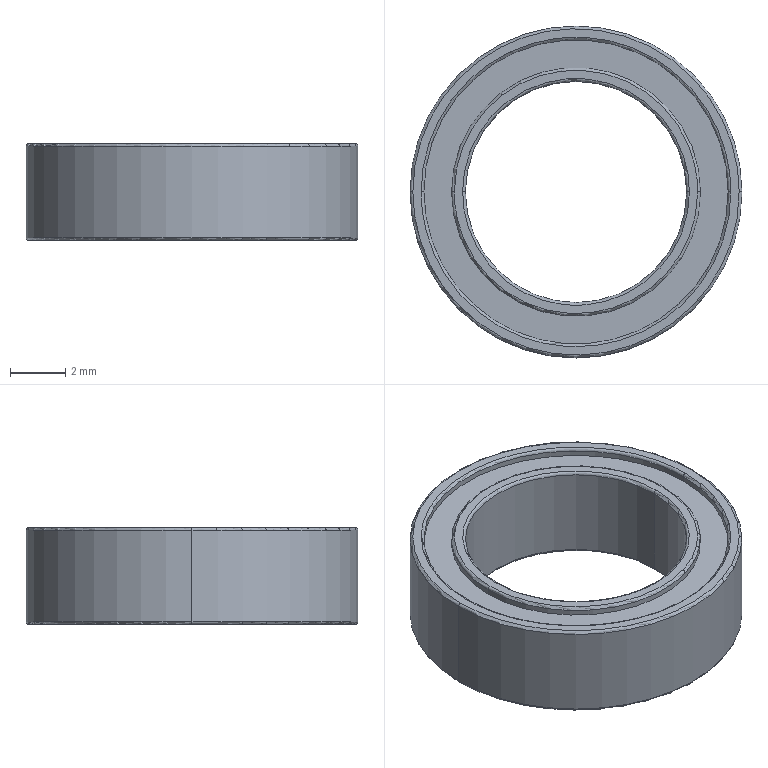Part | NX | features BREP 1 | 1 solid | 34 faces | box 12 x 12 x 3.5 mm | volume 200.575 mm3 | torus 16 | cylinder 12 | plane 6 | commonest cylinder face diameters 9 x4 11 x4 8 x2 12 x2
STEP:
#1=CARTESIAN_POINT('',(-6.,0.,0.1));
#2=VERTEX_POINT('',#1);
#3=CARTESIAN_POINT('',(6.,0.,0.1));
#4=VERTEX_POINT('',#3);
#5=CARTESIAN_POINT('',(0.,0.,0.1));
#6=DIRECTION('',(0.,0.,1.));
#7=DIRECTION('',(-1.,0.,0.));
#8=AXIS2_PLACEMENT_3D('',#5,#6,#7);
#9=CIRCLE('',#8,6.);
#10=EDGE_CURVE('',#2,#4,#9,.T.);
#11=ORIENTED_EDGE('',*,*,#10,.F.);
#12=CARTESIAN_POINT('',(-5.9,0.,0.));
#13=VERTEX_POINT('',#12);
#14=CARTESIAN_POINT('',(-5.9,0.,0.1));
#15=DIRECTION('',(0.,-1.,0.));
#16=DIRECTION('',(-1.,0.,0.));
#17=AXIS2_PLACEMENT_3D('',#14,#15,#16);
#18=CIRCLE('',#17,0.1);
#19=EDGE_CURVE('',#13,#2,#18,.F.);
#20=ORIENTED_EDGE('',*,*,#19,.F.);
#21=CARTESIAN_POINT('',(5.9,0.,0.));
#22=VERTEX_POINT('',#21);
#23=CARTESIAN_POINT('',(-5.9,0.,0.));
#24=CARTESIAN_POINT('',(-5.9,-11.8,0.));
#25=CARTESIAN_POINT('',(5.9,-11.8,0.));
#26=CARTESIAN_POINT('',(5.9,0.,0.));
#27=(BOUNDED_CURVE()B_SPLINE_CURVE(3,(#23,#24,#25,#26),.UNSPECIFIED.,.F.,.F.)B_SPLINE_CURVE_WITH_KNOTS((4,4),(0.,1.),.UNSPECIFIED.)CURVE()GEOMETRIC_REPRESENTATION_ITEM()RATIONAL_B_SPLINE_CURVE((1.,0.3333,0.3333,1.))REPRESENTATION_ITEM(''));
#28=EDGE_CURVE('',#13,#22,#27,.T.);
#29=ORIENTED_EDGE('',*,*,#28,.T.);
#30=CARTESIAN_POINT('',(5.9,0.,0.1));
#31=DIRECTION('',(0.,1.,0.));
#32=DIRECTION('',(1.,0.,0.));
#33=AXIS2_PLACEMENT_3D('',#30,#31,#32);
#34=CIRCLE('',#33,0.1);
#35=EDGE_CURVE('',#22,#4,#34,.F.);
#36=ORIENTED_EDGE('',*,*,#35,.T.);
#37=EDGE_LOOP('',(#11,#20,#29,#36));
#38=FACE_BOUND('',#37,.T.);
#39=CARTESIAN_POINT('',(0.,0.,0.1));
#40=DIRECTION('',(0.,0.,1.));
#41=DIRECTION('',(0.,-1.,0.));
#42=AXIS2_PLACEMENT_3D('',#39,#40,#41);
#43=TOROIDAL_SURFACE('',#42,5.9,0.1);
#44=ADVANCED_FACE('',(#38),#43,.T.);
#45=CARTESIAN_POINT('',(5.9,0.,3.5));
#46=VERTEX_POINT('',#45);
#47=CARTESIAN_POINT('',(-5.9,0.,3.5));
#48=VERTEX_POINT('',#47);
#49=CARTESIAN_POINT('',(5.9,0.,3.5));
#50=CARTESIAN_POINT('',(5.9,-11.8,3.5));
#51=CARTESIAN_POINT('',(-5.9,-11.8,3.5));
#52=CARTESIAN_POINT('',(-5.9,0.,3.5));
#53=(BOUNDED_CURVE()B_SPLINE_CURVE(3,(#49,#50,#51,#52),.UNSPECIFIED.,.F.,.F.)B_SPLINE_CURVE_WITH_KNOTS((4,4),(0.,1.),.UNSPECIFIED.)CURVE()GEOMETRIC_REPRESENTATION_ITEM()RATIONAL_B_SPLINE_CURVE((1.,0.3333,0.3333,1.))REPRESENTATION_ITEM(''));
#54=EDGE_CURVE('',#46,#48,#53,.T.);
#55=ORIENTED_EDGE('',*,*,#54,.T.);
#56=CARTESIAN_POINT('',(-6.,0.,3.4));
#57=VERTEX_POINT('',#56);
#58=CARTESIAN_POINT('',(-5.9,0.,3.4));
#59=DIRECTION('',(0.,-1.,0.));
#60=DIRECTION('',(-1.,0.,0.));
#61=AXIS2_PLACEMENT_3D('',#58,#59,#60);
#62=CIRCLE('',#61,0.1);
#63=EDGE_CURVE('',#57,#48,#62,.F.);
#64=ORIENTED_EDGE('',*,*,#63,.F.);
#65=CARTESIAN_POINT('',(6.,0.,3.4));
#66=VERTEX_POINT('',#65);
#67=CARTESIAN_POINT('',(0.,0.,3.4));
#68=DIRECTION('',(0.,0.,-1.));
#69=DIRECTION('',(-1.,0.,0.));
#70=AXIS2_PLACEMENT_3D('',#67,#68,#69);
#71=CIRCLE('',#70,6.);
#72=EDGE_CURVE('',#66,#57,#71,.T.);
#73=ORIENTED_EDGE('',*,*,#72,.F.);
#74=CARTESIAN_POINT('',(5.9,0.,3.4));
#75=DIRECTION('',(0.,1.,0.));
#76=DIRECTION('',(1.,0.,0.));
#77=AXIS2_PLACEMENT_3D('',#74,#75,#76);
#78=CIRCLE('',#77,0.1);
#79=EDGE_CURVE('',#66,#46,#78,.F.);
#80=ORIENTED_EDGE('',*,*,#79,.T.);
#81=EDGE_LOOP('',(#55,#64,#73,#80));
#82=FACE_BOUND('',#81,.T.);
#83=CARTESIAN_POINT('',(0.,0.,3.4));
#84=DIRECTION('',(0.,0.,1.));
#85=DIRECTION('',(0.,-1.,0.));
#86=AXIS2_PLACEMENT_3D('',#83,#84,#85);
#87=TOROIDAL_SURFACE('',#86,5.9,0.1);
#88=ADVANCED_FACE('',(#82),#87,.T.);
#89=CARTESIAN_POINT('',(5.6,0.,0.));
#90=VERTEX_POINT('',#89);
#91=CARTESIAN_POINT('',(-5.6,0.,0.));
#92=VERTEX_POINT('',#91);
#93=CARTESIAN_POINT('',(5.6,0.,0.));
#94=CARTESIAN_POINT('',(5.6,-11.2,0.));
#95=CARTESIAN_POINT('',(-5.6,-11.2,0.));
#96=CARTESIAN_POINT('',(-5.6,0.,0.));
#97=(BOUNDED_CURVE()B_SPLINE_CURVE(3,(#93,#94,#95,#96),.UNSPECIFIED.,.F.,.F.)B_SPLINE_CURVE_WITH_KNOTS((4,4),(0.,1.),.UNSPECIFIED.)CURVE()GEOMETRIC_REPRESENTATION_ITEM()RATIONAL_B_SPLINE_CURVE((1.,0.3333,0.3333,1.))REPRESENTATION_ITEM(''));
#98=EDGE_CURVE('',#90,#92,#97,.T.);
#99=ORIENTED_EDGE('',*,*,#98,.T.);
#100=CARTESIAN_POINT('',(-5.5,0.,0.1));
#101=VERTEX_POINT('',#100);
#102=CARTESIAN_POINT('',(-5.6,0.,0.1));
#103=DIRECTION('',(0.,-1.,0.));
#104=DIRECTION('',(-1.,0.,0.));
#105=AXIS2_PLACEMENT_3D('',#102,#103,#104);
#106=CIRCLE('',#105,0.1);
#107=EDGE_CURVE('',#101,#92,#106,.F.);
#108=ORIENTED_EDGE('',*,*,#107,.F.);
#109=CARTESIAN_POINT('',(5.5,0.,0.1));
#110=VERTEX_POINT('',#109);
#111=CARTESIAN_POINT('',(0.,0.,0.1));
#112=DIRECTION('',(0.,0.,1.));
#113=DIRECTION('',(1.,0.,0.));
#114=AXIS2_PLACEMENT_3D('',#111,#112,#113);
#115=CIRCLE('',#114,5.5);
#116=EDGE_CURVE('',#101,#110,#115,.T.);
#117=ORIENTED_EDGE('',*,*,#116,.T.);
#118=CARTESIAN_POINT('',(5.6,0.,0.1));
#119=DIRECTION('',(0.,1.,0.));
#120=DIRECTION('',(1.,0.,0.));
#121=AXIS2_PLACEMENT_3D('',#118,#119,#120);
#122=CIRCLE('',#121,0.1);
#123=EDGE_CURVE('',#110,#90,#122,.F.);
#124=ORIENTED_EDGE('',*,*,#123,.T.);
#125=EDGE_LOOP('',(#99,#108,#117,#124));
#126=FACE_BOUND('',#125,.T.);
#127=CARTESIAN_POINT('',(0.,0.,0.1));
#128=DIRECTION('',(0.,0.,1.));
#129=DIRECTION('',(1.,0.,0.));
#130=AXIS2_PLACEMENT_3D('',#127,#128,#129);
#131=TOROIDAL_SURFACE('',#130,5.6,0.1);
#132=ADVANCED_FACE('',(#126),#131,.T.);
#133=CARTESIAN_POINT('',(5.5,0.,3.4));
#134=VERTEX_POINT('',#133);
#135=CARTESIAN_POINT('',(-5.5,0.,3.4));
#136=VERTEX_POINT('',#135);
#137=CARTESIAN_POINT('',(0.,0.,3.4));
#138=DIRECTION('',(0.,0.,-1.));
#139=DIRECTION('',(1.,0.,0.));
#140=AXIS2_PLACEMENT_3D('',#137,#138,#139);
#141=CIRCLE('',#140,5.5);
#142=EDGE_CURVE('',#134,#136,#141,.T.);
#143=ORIENTED_EDGE('',*,*,#142,.T.);
#144=CARTESIAN_POINT('',(-5.6,0.,3.5));
#145=VERTEX_POINT('',#144);
#146=CARTESIAN_POINT('',(-5.6,0.,3.4));
#147=DIRECTION('',(0.,-1.,0.));
#148=DIRECTION('',(-1.,0.,0.));
#149=AXIS2_PLACEMENT_3D('',#146,#147,#148);
#150=CIRCLE('',#149,0.1);
#151=EDGE_CURVE('',#145,#136,#150,.F.);
#152=ORIENTED_EDGE('',*,*,#151,.F.);
#153=CARTESIAN_POINT('',(5.6,0.,3.5));
#154=VERTEX_POINT('',#153);
#155=CARTESIAN_POINT('',(5.6,0.,3.5));
#156=CARTESIAN_POINT('',(5.6,-0.1713,3.5));
#157=CARTESIAN_POINT('',(5.588,-0.4272,3.5));
#158=CARTESIAN_POINT('',(5.554,-0.7238,3.5));
#159=CARTESIAN_POINT('',(5.532,-0.8716,3.5));
#160=CARTESIAN_POINT('',(5.521,-0.9348,3.5));
#161=CARTESIAN_POINT('',(5.514,-0.9769,3.5));
#162=CARTESIAN_POINT('',(5.511,-0.9967,3.5));
#163=CARTESIAN_POINT('',(5.474,-1.197,3.5));
#164=CARTESIAN_POINT('',(5.411,-1.462,3.5));
#165=CARTESIAN_POINT('',(5.316,-1.763,3.5));
#166=CARTESIAN_POINT('',(5.271,-1.892,3.5));
#167=CARTESIAN_POINT('',(5.24,-1.977,3.5));
#168=CARTESIAN_POINT('',(5.224,-2.017,3.5));
#169=CARTESIAN_POINT('',(5.137,-2.237,3.5));
#170=CARTESIAN_POINT('',(5.02,-2.494,3.5));
#171=CARTESIAN_POINT('',(4.884,-2.742,3.5));
#172=CARTESIAN_POINT('',(4.789,-2.905,3.5));
#173=CARTESIAN_POINT('',(4.74,-2.984,3.5));
#174=CARTESIAN_POINT('',(4.476,-3.388,3.5));
#175=CARTESIAN_POINT('',(4.233,-3.687,3.5));
#176=CARTESIAN_POINT('',(3.823,-4.096,3.5));
#177=CARTESIAN_POINT('',(3.609,-4.29,3.5));
#178=CARTESIAN_POINT('',(3.38,-4.466,3.5));
#179=CARTESIAN_POINT('',(3.225,-4.579,3.5));
#180=CARTESIAN_POINT('',(3.143,-4.635,3.5));
#181=CARTESIAN_POINT('',(2.906,-4.791,3.5));
#182=CARTESIAN_POINT('',(2.662,-4.933,3.5));
#183=CARTESIAN_POINT('',(2.366,-5.077,3.5));
#184=CARTESIAN_POINT('',(2.236,-5.134,3.5));
#185=CARTESIAN_POINT('',(2.149,-5.171,3.5));
#186=CARTESIAN_POINT('',(2.104,-5.19,3.5));
#187=CARTESIAN_POINT('',(1.893,-5.274,3.5));
#188=CARTESIAN_POINT('',(1.636,-5.361,3.5));
#189=CARTESIAN_POINT('',(1.33,-5.441,3.5));
#190=CARTESIAN_POINT('',(1.175,-5.476,3.5));
#191=CARTESIAN_POINT('',(1.108,-5.489,3.5));
#192=CARTESIAN_POINT('',(1.064,-5.498,3.5));
#193=CARTESIAN_POINT('',(1.04,-5.503,3.5));
#194=CARTESIAN_POINT('',(0.6825,-5.569,3.5));
#195=CARTESIAN_POINT('',(0.3422,-5.6,3.5));
#196=CARTESIAN_POINT('',(-0.1711,-5.6,3.5));
#197=CARTESIAN_POINT('',(-0.4268,-5.588,3.5));
#198=CARTESIAN_POINT('',(-0.7234,-5.554,3.5));
#199=CARTESIAN_POINT('',(-0.8713,-5.532,3.5));
#200=CARTESIAN_POINT('',(-0.9347,-5.521,3.5));
#201=CARTESIAN_POINT('',(-0.9768,-5.514,3.5));
#202=CARTESIAN_POINT('',(-0.9967,-5.511,3.5));
#203=CARTESIAN_POINT('',(-1.197,-5.474,3.5));
#204=CARTESIAN_POINT('',(-1.462,-5.411,3.5));
#205=CARTESIAN_POINT('',(-1.763,-5.316,3.5));
#206=CARTESIAN_POINT('',(-1.892,-5.271,3.5));
#207=CARTESIAN_POINT('',(-1.977,-5.24,3.5));
#208=CARTESIAN_POINT('',(-2.017,-5.224,3.5));
#209=CARTESIAN_POINT('',(-2.237,-5.137,3.5));
#210=CARTESIAN_POINT('',(-2.494,-5.02,3.5));
#211=CARTESIAN_POINT('',(-2.742,-4.884,3.5));
#212=CARTESIAN_POINT('',(-2.905,-4.789,3.5));
#213=CARTESIAN_POINT('',(-2.984,-4.74,3.5));
#214=CARTESIAN_POINT('',(-3.388,-4.476,3.5));
#215=CARTESIAN_POINT('',(-3.687,-4.233,3.5));
#216=CARTESIAN_POINT('',(-4.096,-3.823,3.5));
#217=CARTESIAN_POINT('',(-4.29,-3.609,3.5));
#218=CARTESIAN_POINT('',(-4.466,-3.38,3.5));
#219=CARTESIAN_POINT('',(-4.579,-3.225,3.5));
#220=CARTESIAN_POINT('',(-4.635,-3.143,3.5));
#221=CARTESIAN_POINT('',(-4.791,-2.906,3.5));
#222=CARTESIAN_POINT('',(-4.933,-2.662,3.5));
#223=CARTESIAN_POINT('',(-5.077,-2.366,3.5));
#224=CARTESIAN_POINT('',(-5.134,-2.236,3.5));
#225=CARTESIAN_POINT('',(-5.171,-2.149,3.5));
#226=CARTESIAN_POINT('',(-5.19,-2.104,3.5));
#227=CARTESIAN_POINT('',(-5.274,-1.893,3.5));
#228=CARTESIAN_POINT('',(-5.361,-1.636,3.5));
#229=CARTESIAN_POINT('',(-5.441,-1.33,3.5));
#230=CARTESIAN_POINT('',(-5.476,-1.175,3.5));
#231=CARTESIAN_POINT('',(-5.489,-1.108,3.5));
#232=CARTESIAN_POINT('',(-5.498,-1.064,3.5));
#233=CARTESIAN_POINT('',(-5.503,-1.04,3.5));
#234=CARTESIAN_POINT('',(-5.569,-0.6827,3.5));
#235=CARTESIAN_POINT('',(-5.6,-0.3431,3.5));
#236=CARTESIAN_POINT('',(-5.6,0.,3.5));
#237=B_SPLINE_CURVE_WITH_KNOTS('',3,(#155,#156,#157,#158,#159,#160,#161,#162,#163,#164,#165,#166,#167,#168,#169,#170,#171,#172,#173,#174,#175,#176,#177,#178,#179,#180,#181,#182,#183,#184,#185,#186,#187,#188,#189,#190,#191,#192,#193,#194,#195,#196,#197,#198,#199,#200,#201,#202,#203,#204,#205,#206,#207,#208,#209,#210,#211,#212,#213,#214,#215,#216,#217,#218,#219,#220,#221,#222,#223,#224,#225,#226,#227,#228,#229,#230,#231,#232,#233,#234,#235,#236),.UNSPECIFIED.,.F.,.F.,(4,1,1,1,2,2,1,1,2,2,1,2,2,2,1,2,2,1,1,2,2,1,1,1,2,2,2,1,1,1,2,2,1,1,2,2,1,2,2,2,1,2,2,1,1,2,2,1,1,1,2,2,4),(0.,0.03125,0.04688,0.05469,0.05859,0.0625,0.09375,0.1094,0.1172,0.125,0.1562,0.1719,0.1875,0.25,0.2812,0.2969,0.3125,0.3438,0.3594,0.3672,0.375,0.4062,0.4219,0.4297,0.4336,0.4375,0.5,0.5312,0.5469,0.5547,0.5586,0.5625,0.5938,0.6094,0.6172,0.625,0.6562,0.6719,0.6875,0.75,0.7812,0.7969,0.8125,0.8438,0.8594,0.8672,0.875,0.9062,0.9219,0.9297,0.9336,0.9375,1.),.UNSPECIFIED.);
#238=EDGE_CURVE('',#154,#145,#237,.T.);
#239=ORIENTED_EDGE('',*,*,#238,.F.);
#240=CARTESIAN_POINT('',(5.6,0.,3.4));
#241=DIRECTION('',(0.,1.,0.));
#242=DIRECTION('',(1.,0.,0.));
#243=AXIS2_PLACEMENT_3D('',#240,#241,#242);
#244=CIRCLE('',#243,0.1);
#245=EDGE_CURVE('',#154,#134,#244,.F.);
#246=ORIENTED_EDGE('',*,*,#245,.T.);
#247=EDGE_LOOP('',(#143,#152,#239,#246));
#248=FACE_BOUND('',#247,.T.);
#249=CARTESIAN_POINT('',(0.,0.,3.4));
#250=DIRECTION('',(0.,0.,1.));
#251=DIRECTION('',(0.,-1.,0.));
#252=AXIS2_PLACEMENT_3D('',#249,#250,#251);
#253=TOROIDAL_SURFACE('',#252,5.6,0.1);
#254=ADVANCED_FACE('',(#248),#253,.T.);
#255=CARTESIAN_POINT('',(-4.4,0.,0.));
#256=VERTEX_POINT('',#255);
#257=CARTESIAN_POINT('',(4.4,0.,0.));
#258=VERTEX_POINT('',#257);
#259=CARTESIAN_POINT('',(-4.4,0.,0.));
#260=CARTESIAN_POINT('',(-4.4,-8.8,0.));
#261=CARTESIAN_POINT('',(4.4,-8.8,0.));
#262=CARTESIAN_POINT('',(4.4,0.,0.));
#263=(BOUNDED_CURVE()B_SPLINE_CURVE(3,(#259,#260,#261,#262),.UNSPECIFIED.,.F.,.F.)B_SPLINE_CURVE_WITH_KNOTS((4,4),(0.,1.),.UNSPECIFIED.)CURVE()GEOMETRIC_REPRESENTATION_ITEM()RATIONAL_B_SPLINE_CURVE((1.,0.3333,0.3333,1.))REPRESENTATION_ITEM(''));
#264=EDGE_CURVE('',#256,#258,#263,.T.);
#265=ORIENTED_EDGE('',*,*,#264,.T.);
#266=CARTESIAN_POINT('',(4.5,0.,0.1));
#267=VERTEX_POINT('',#266);
#268=CARTESIAN_POINT('',(4.4,0.,0.1));
#269=DIRECTION('',(0.,-1.,0.));
#270=DIRECTION('',(1.,0.,0.));
#271=AXIS2_PLACEMENT_3D('',#268,#269,#270);
#272=CIRCLE('',#271,0.1);
#273=EDGE_CURVE('',#258,#267,#272,.T.);
#274=ORIENTED_EDGE('',*,*,#273,.T.);
#275=CARTESIAN_POINT('',(-4.5,0.,0.1));
#276=VERTEX_POINT('',#275);
#277=CARTESIAN_POINT('',(0.,0.,0.1));
#278=DIRECTION('',(0.,0.,1.));
#279=DIRECTION('',(1.,0.,0.));
#280=AXIS2_PLACEMENT_3D('',#277,#278,#279);
#281=CIRCLE('',#280,4.5);
#282=EDGE_CURVE('',#276,#267,#281,.T.);
#283=ORIENTED_EDGE('',*,*,#282,.F.);
#284=CARTESIAN_POINT('',(-4.4,0.,0.1));
#285=DIRECTION('',(0.,1.,0.));
#286=DIRECTION('',(-1.,0.,0.));
#287=AXIS2_PLACEMENT_3D('',#284,#285,#286);
#288=CIRCLE('',#287,0.1);
#289=EDGE_CURVE('',#256,#276,#288,.T.);
#290=ORIENTED_EDGE('',*,*,#289,.F.);
#291=EDGE_LOOP('',(#265,#274,#283,#290));
#292=FACE_BOUND('',#291,.T.);
#293=CARTESIAN_POINT('',(0.,0.,0.1));
#294=DIRECTION('',(0.,0.,1.));
#295=DIRECTION('',(0.,-1.,0.));
#296=AXIS2_PLACEMENT_3D('',#293,#294,#295);
#297=TOROIDAL_SURFACE('',#296,4.4,0.1);
#298=ADVANCED_FACE('',(#292),#297,.T.);
#299=CARTESIAN_POINT('',(4.4,0.,3.5));
#300=VERTEX_POINT('',#299);
#301=CARTESIAN_POINT('',(-4.4,0.,3.5));
#302=VERTEX_POINT('',#301);
#303=CARTESIAN_POINT('',(4.4,0.,3.5));
#304=CARTESIAN_POINT('',(4.4,-8.8,3.5));
#305=CARTESIAN_POINT('',(-4.4,-8.8,3.5));
#306=CARTESIAN_POINT('',(-4.4,0.,3.5));
#307=(BOUNDED_CURVE()B_SPLINE_CURVE(3,(#303,#304,#305,#306),.UNSPECIFIED.,.F.,.F.)B_SPLINE_CURVE_WITH_KNOTS((4,4),(0.,1.),.UNSPECIFIED.)CURVE()GEOMETRIC_REPRESENTATION_ITEM()RATIONAL_B_SPLINE_CURVE((1.,0.3333,0.3333,1.))REPRESENTATION_ITEM(''));
#308=EDGE_CURVE('',#300,#302,#307,.T.);
#309=ORIENTED_EDGE('',*,*,#308,.T.);
#310=CARTESIAN_POINT('',(-4.5,0.,3.4));
#311=VERTEX_POINT('',#310);
#312=CARTESIAN_POINT('',(-4.4,0.,3.4));
#313=DIRECTION('',(0.,-1.,0.));
#314=DIRECTION('',(-1.,0.,0.));
#315=AXIS2_PLACEMENT_3D('',#312,#313,#314);
#316=CIRCLE('',#315,0.1);
#317=EDGE_CURVE('',#311,#302,#316,.F.);
#318=ORIENTED_EDGE('',*,*,#317,.F.);
#319=CARTESIAN_POINT('',(4.5,0.,3.4));
#320=VERTEX_POINT('',#319);
#321=CARTESIAN_POINT('',(0.,0.,3.4));
#322=DIRECTION('',(0.,0.,-1.));
#323=DIRECTION('',(-1.,0.,0.));
#324=AXIS2_PLACEMENT_3D('',#321,#322,#323);
#325=CIRCLE('',#324,4.5);
#326=EDGE_CURVE('',#320,#311,#325,.T.);
#327=ORIENTED_EDGE('',*,*,#326,.F.);
#328=CARTESIAN_POINT('',(4.4,0.,3.4));
#329=DIRECTION('',(0.,1.,0.));
#330=DIRECTION('',(1.,0.,0.));
#331=AXIS2_PLACEMENT_3D('',#328,#329,#330);
#332=CIRCLE('',#331,0.1);
#333=EDGE_CURVE('',#320,#300,#332,.F.);
#334=ORIENTED_EDGE('',*,*,#333,.T.);
#335=EDGE_LOOP('',(#309,#318,#327,#334));
#336=FACE_BOUND('',#335,.T.);
#337=CARTESIAN_POINT('',(0.,0.,3.4));
#338=DIRECTION('',(0.,0.,1.));
#339=DIRECTION('',(0.,-1.,0.));
#340=AXIS2_PLACEMENT_3D('',#337,#338,#339);
#341=TOROIDAL_SURFACE('',#340,4.4,0.1);
#342=ADVANCED_FACE('',(#336),#341,.T.);
#343=CARTESIAN_POINT('',(-4.,0.,0.1));
#344=VERTEX_POINT('',#343);
#345=CARTESIAN_POINT('',(4.,0.,0.1));
#346=VERTEX_POINT('',#345);
#347=CARTESIAN_POINT('',(0.,0.,0.1));
#348=DIRECTION('',(0.,0.,1.));
#349=DIRECTION('',(-1.,0.,0.));
#350=AXIS2_PLACEMENT_3D('',#347,#348,#349);
#351=CIRCLE('',#350,4.);
#352=EDGE_CURVE('',#344,#346,#351,.T.);
#353=ORIENTED_EDGE('',*,*,#352,.T.);
#354=CARTESIAN_POINT('',(4.1,0.,0.));
#355=VERTEX_POINT('',#354);
#356=CARTESIAN_POINT('',(4.1,0.,0.1));
#357=DIRECTION('',(0.,-1.,0.));
#358=DIRECTION('',(1.,0.,0.));
#359=AXIS2_PLACEMENT_3D('',#356,#357,#358);
#360=CIRCLE('',#359,0.1);
#361=EDGE_CURVE('',#346,#355,#360,.T.);
#362=ORIENTED_EDGE('',*,*,#361,.T.);
#363=CARTESIAN_POINT('',(-4.1,0.,0.));
#364=VERTEX_POINT('',#363);
#365=CARTESIAN_POINT('',(-4.1,0.,0.));
#366=CARTESIAN_POINT('',(-4.1,-0.2608,0.));
#367=CARTESIAN_POINT('',(-4.064,-0.645,0.));
#368=CARTESIAN_POINT('',(-3.959,-1.081,0.));
#369=CARTESIAN_POINT('',(-3.891,-1.296,0.));
#370=CARTESIAN_POINT('',(-3.858,-1.388,0.));
#371=CARTESIAN_POINT('',(-3.836,-1.449,0.));
#372=CARTESIAN_POINT('',(-3.825,-1.477,0.));
#373=CARTESIAN_POINT('',(-3.761,-1.638,0.));
#374=CARTESIAN_POINT('',(-3.675,-1.826,0.));
#375=CARTESIAN_POINT('',(-3.576,-2.007,0.));
#376=CARTESIAN_POINT('',(-3.506,-2.127,0.));
#377=CARTESIAN_POINT('',(-3.47,-2.184,0.));
#378=CARTESIAN_POINT('',(-3.277,-2.48,0.));
#379=CARTESIAN_POINT('',(-3.099,-2.699,0.));
#380=CARTESIAN_POINT('',(-2.799,-2.999,0.));
#381=CARTESIAN_POINT('',(-2.642,-3.141,0.));
#382=CARTESIAN_POINT('',(-2.475,-3.27,0.));
#383=CARTESIAN_POINT('',(-2.361,-3.353,0.));
#384=CARTESIAN_POINT('',(-2.301,-3.394,0.));
#385=CARTESIAN_POINT('',(-2.128,-3.507,0.));
#386=CARTESIAN_POINT('',(-1.949,-3.612,0.));
#387=CARTESIAN_POINT('',(-1.732,-3.717,0.));
#388=CARTESIAN_POINT('',(-1.637,-3.759,0.));
#389=CARTESIAN_POINT('',(-1.573,-3.786,0.));
#390=CARTESIAN_POINT('',(-1.539,-3.8,0.));
#391=CARTESIAN_POINT('',(-1.025,-4.004,0.));
#392=CARTESIAN_POINT('',(-0.521,-4.1,0.));
#393=CARTESIAN_POINT('',(0.2605,-4.1,0.));
#394=CARTESIAN_POINT('',(0.6445,-4.064,0.));
#395=CARTESIAN_POINT('',(1.081,-3.959,0.));
#396=CARTESIAN_POINT('',(1.296,-3.891,0.));
#397=CARTESIAN_POINT('',(1.388,-3.858,0.));
#398=CARTESIAN_POINT('',(1.448,-3.836,0.));
#399=CARTESIAN_POINT('',(1.477,-3.825,0.));
#400=CARTESIAN_POINT('',(1.638,-3.761,0.));
#401=CARTESIAN_POINT('',(1.826,-3.675,0.));
#402=CARTESIAN_POINT('',(2.007,-3.576,0.));
#403=CARTESIAN_POINT('',(2.127,-3.506,0.));
#404=CARTESIAN_POINT('',(2.184,-3.47,0.));
#405=CARTESIAN_POINT('',(2.48,-3.277,0.));
#406=CARTESIAN_POINT('',(2.699,-3.099,0.));
#407=CARTESIAN_POINT('',(2.999,-2.799,0.));
#408=CARTESIAN_POINT('',(3.141,-2.642,0.));
#409=CARTESIAN_POINT('',(3.27,-2.475,0.));
#410=CARTESIAN_POINT('',(3.353,-2.361,0.));
#411=CARTESIAN_POINT('',(3.394,-2.301,0.));
#412=CARTESIAN_POINT('',(3.507,-2.128,0.));
#413=CARTESIAN_POINT('',(3.612,-1.949,0.));
#414=CARTESIAN_POINT('',(3.717,-1.732,0.));
#415=CARTESIAN_POINT('',(3.759,-1.637,0.));
#416=CARTESIAN_POINT('',(3.786,-1.573,0.));
#417=CARTESIAN_POINT('',(3.8,-1.539,0.));
#418=CARTESIAN_POINT('',(4.004,-1.025,0.));
#419=CARTESIAN_POINT('',(4.1,-0.5219,0.));
#420=CARTESIAN_POINT('',(4.1,0.,0.));
#421=B_SPLINE_CURVE_WITH_KNOTS('',3,(#365,#366,#367,#368,#369,#370,#371,#372,#373,#374,#375,#376,#377,#378,#379,#380,#381,#382,#383,#384,#385,#386,#387,#388,#389,#390,#391,#392,#393,#394,#395,#396,#397,#398,#399,#400,#401,#402,#403,#404,#405,#406,#407,#408,#409,#410,#411,#412,#413,#414,#415,#416,#417,#418,#419,#420),.UNSPECIFIED.,.F.,.F.,(4,1,1,1,2,2,1,2,2,2,1,2,2,1,1,2,2,2,1,1,1,2,2,1,2,2,2,1,2,2,1,1,2,2,4),(0.,0.0625,0.09375,0.1094,0.1172,0.125,0.1562,0.1719,0.1875,0.25,0.2812,0.2969,0.3125,0.3438,0.3594,0.3672,0.375,0.5,0.5625,0.5938,0.6094,0.6172,0.625,0.6562,0.6719,0.6875,0.75,0.7812,0.7969,0.8125,0.8438,0.8594,0.8672,0.875,1.),.UNSPECIFIED.);
#422=EDGE_CURVE('',#364,#355,#421,.T.);
#423=ORIENTED_EDGE('',*,*,#422,.F.);
#424=CARTESIAN_POINT('',(-4.1,0.,0.1));
#425=DIRECTION('',(0.,1.,0.));
#426=DIRECTION('',(-1.,0.,0.));
#427=AXIS2_PLACEMENT_3D('',#424,#425,#426);
#428=CIRCLE('',#427,0.1);
#429=EDGE_CURVE('',#344,#364,#428,.T.);
#430=ORIENTED_EDGE('',*,*,#429,.F.);
#431=EDGE_LOOP('',(#353,#362,#423,#430));
#432=FACE_BOUND('',#431,.T.);
#433=CARTESIAN_POINT('',(0.,0.,0.1));
#434=DIRECTION('',(0.,0.,1.));
#435=DIRECTION('',(0.,-1.,0.));
#436=AXIS2_PLACEMENT_3D('',#433,#434,#435);
#437=TOROIDAL_SURFACE('',#436,4.1,0.1);
#438=ADVANCED_FACE('',(#432),#437,.T.);
#439=CARTESIAN_POINT('',(4.,0.,3.4));
#440=VERTEX_POINT('',#439);
#441=CARTESIAN_POINT('',(-4.,0.,3.4));
#442=VERTEX_POINT('',#441);
#443=CARTESIAN_POINT('',(0.,0.,3.4));
#444=DIRECTION('',(0.,0.,-1.));
#445=DIRECTION('',(1.,0.,0.));
#446=AXIS2_PLACEMENT_3D('',#443,#444,#445);
#447=CIRCLE('',#446,4.);
#448=EDGE_CURVE('',#440,#442,#447,.T.);
#449=ORIENTED_EDGE('',*,*,#448,.T.);
#450=CARTESIAN_POINT('',(-4.1,0.,3.5));
#451=VERTEX_POINT('',#450);
#452=CARTESIAN_POINT('',(-4.1,0.,3.4));
#453=DIRECTION('',(0.,-1.,0.));
#454=DIRECTION('',(-1.,0.,0.));
#455=AXIS2_PLACEMENT_3D('',#452,#453,#454);
#456=CIRCLE('',#455,0.1);
#457=EDGE_CURVE('',#451,#442,#456,.F.);
#458=ORIENTED_EDGE('',*,*,#457,.F.);
#459=CARTESIAN_POINT('',(4.1,0.,3.5));
#460=VERTEX_POINT('',#459);
#461=CARTESIAN_POINT('',(4.1,0.,3.5));
#462=CARTESIAN_POINT('',(4.1,-0.2608,3.5));
#463=CARTESIAN_POINT('',(4.064,-0.645,3.5));
#464=CARTESIAN_POINT('',(3.959,-1.081,3.5));
#465=CARTESIAN_POINT('',(3.891,-1.296,3.5));
#466=CARTESIAN_POINT('',(3.858,-1.388,3.5));
#467=CARTESIAN_POINT('',(3.836,-1.449,3.5));
#468=CARTESIAN_POINT('',(3.825,-1.477,3.5));
#469=CARTESIAN_POINT('',(3.761,-1.638,3.5));
#470=CARTESIAN_POINT('',(3.675,-1.826,3.5));
#471=CARTESIAN_POINT('',(3.576,-2.007,3.5));
#472=CARTESIAN_POINT('',(3.506,-2.127,3.5));
#473=CARTESIAN_POINT('',(3.47,-2.184,3.5));
#474=CARTESIAN_POINT('',(3.277,-2.48,3.5));
#475=CARTESIAN_POINT('',(3.099,-2.699,3.5));
#476=CARTESIAN_POINT('',(2.799,-2.999,3.5));
#477=CARTESIAN_POINT('',(2.642,-3.141,3.5));
#478=CARTESIAN_POINT('',(2.475,-3.27,3.5));
#479=CARTESIAN_POINT('',(2.361,-3.353,3.5));
#480=CARTESIAN_POINT('',(2.301,-3.394,3.5));
#481=CARTESIAN_POINT('',(2.128,-3.507,3.5));
#482=CARTESIAN_POINT('',(1.949,-3.612,3.5));
#483=CARTESIAN_POINT('',(1.732,-3.717,3.5));
#484=CARTESIAN_POINT('',(1.637,-3.759,3.5));
#485=CARTESIAN_POINT('',(1.573,-3.786,3.5));
#486=CARTESIAN_POINT('',(1.539,-3.8,3.5));
#487=CARTESIAN_POINT('',(1.025,-4.004,3.5));
#488=CARTESIAN_POINT('',(0.521,-4.1,3.5));
#489=CARTESIAN_POINT('',(-0.2605,-4.1,3.5));
#490=CARTESIAN_POINT('',(-0.6445,-4.064,3.5));
#491=CARTESIAN_POINT('',(-1.081,-3.959,3.5));
#492=CARTESIAN_POINT('',(-1.296,-3.891,3.5));
#493=CARTESIAN_POINT('',(-1.388,-3.858,3.5));
#494=CARTESIAN_POINT('',(-1.448,-3.836,3.5));
#495=CARTESIAN_POINT('',(-1.477,-3.825,3.5));
#496=CARTESIAN_POINT('',(-1.638,-3.761,3.5));
#497=CARTESIAN_POINT('',(-1.826,-3.675,3.5));
#498=CARTESIAN_POINT('',(-2.007,-3.576,3.5));
#499=CARTESIAN_POINT('',(-2.127,-3.506,3.5));
#500=CARTESIAN_POINT('',(-2.184,-3.47,3.5));
#501=CARTESIAN_POINT('',(-2.48,-3.277,3.5));
#502=CARTESIAN_POINT('',(-2.699,-3.099,3.5));
#503=CARTESIAN_POINT('',(-2.999,-2.799,3.5));
#504=CARTESIAN_POINT('',(-3.141,-2.642,3.5));
#505=CARTESIAN_POINT('',(-3.27,-2.475,3.5));
#506=CARTESIAN_POINT('',(-3.353,-2.361,3.5));
#507=CARTESIAN_POINT('',(-3.394,-2.301,3.5));
#508=CARTESIAN_POINT('',(-3.507,-2.128,3.5));
#509=CARTESIAN_POINT('',(-3.612,-1.949,3.5));
#510=CARTESIAN_POINT('',(-3.717,-1.732,3.5));
#511=CARTESIAN_POINT('',(-3.759,-1.637,3.5));
#512=CARTESIAN_POINT('',(-3.786,-1.573,3.5));
#513=CARTESIAN_POINT('',(-3.8,-1.539,3.5));
#514=CARTESIAN_POINT('',(-4.004,-1.025,3.5));
#515=CARTESIAN_POINT('',(-4.1,-0.5219,3.5));
#516=CARTESIAN_POINT('',(-4.1,0.,3.5));
#517=B_SPLINE_CURVE_WITH_KNOTS('',3,(#461,#462,#463,#464,#465,#466,#467,#468,#469,#470,#471,#472,#473,#474,#475,#476,#477,#478,#479,#480,#481,#482,#483,#484,#485,#486,#487,#488,#489,#490,#491,#492,#493,#494,#495,#496,#497,#498,#499,#500,#501,#502,#503,#504,#505,#506,#507,#508,#509,#510,#511,#512,#513,#514,#515,#516),.UNSPECIFIED.,.F.,.F.,(4,1,1,1,2,2,1,2,2,2,1,2,2,1,1,2,2,2,1,1,1,2,2,1,2,2,2,1,2,2,1,1,2,2,4),(0.,0.0625,0.09375,0.1094,0.1172,0.125,0.1562,0.1719,0.1875,0.25,0.2812,0.2969,0.3125,0.3438,0.3594,0.3672,0.375,0.5,0.5625,0.5938,0.6094,0.6172,0.625,0.6562,0.6719,0.6875,0.75,0.7812,0.7969,0.8125,0.8438,0.8594,0.8672,0.875,1.),.UNSPECIFIED.);
#518=EDGE_CURVE('',#460,#451,#517,.T.);
#519=ORIENTED_EDGE('',*,*,#518,.F.);
#520=CARTESIAN_POINT('',(4.1,0.,3.4));
#521=DIRECTION('',(0.,1.,0.));
#522=DIRECTION('',(1.,0.,0.));
#523=AXIS2_PLACEMENT_3D('',#520,#521,#522);
#524=CIRCLE('',#523,0.1);
#525=EDGE_CURVE('',#460,#440,#524,.F.);
#526=ORIENTED_EDGE('',*,*,#525,.T.);
#527=EDGE_LOOP('',(#449,#458,#519,#526));
#528=FACE_BOUND('',#527,.T.);
#529=CARTESIAN_POINT('',(0.,0.,3.4));
#530=DIRECTION('',(0.,0.,1.));
#531=DIRECTION('',(0.,-1.,0.));
#532=AXIS2_PLACEMENT_3D('',#529,#530,#531);
#533=TOROIDAL_SURFACE('',#532,4.1,0.1);
#534=ADVANCED_FACE('',(#528),#533,.T.);
#535=CARTESIAN_POINT('',(0.,0.,3.4));
#536=DIRECTION('',(0.,0.,-1.));
#537=DIRECTION('',(-1.,0.,0.));
#538=AXIS2_PLACEMENT_3D('',#535,#536,#537);
#539=CIRCLE('',#538,6.);
#540=EDGE_CURVE('',#57,#66,#539,.T.);
#541=ORIENTED_EDGE('',*,*,#540,.T.);
#542=CARTESIAN_POINT('',(6.,0.,3.5));
#543=DIRECTION('',(0.,0.,-1.));
#544=VECTOR('',#543,1000.);
#545=LINE('',#542,#544);
#546=EDGE_CURVE('',#66,#4,#545,.T.);
#547=ORIENTED_EDGE('',*,*,#546,.T.);
#548=CARTESIAN_POINT('',(0.,0.,0.1));
#549=DIRECTION('',(0.,0.,1.));
#550=DIRECTION('',(-1.,0.,0.));
#551=AXIS2_PLACEMENT_3D('',#548,#549,#550);
#552=CIRCLE('',#551,6.);
#553=EDGE_CURVE('',#4,#2,#552,.T.);
#554=ORIENTED_EDGE('',*,*,#553,.T.);
#555=CARTESIAN_POINT('',(-6.,0.,3.5));
#556=DIRECTION('',(0.,0.,-1.));
#557=VECTOR('',#556,1000.);
#558=LINE('',#555,#557);
#559=EDGE_CURVE('',#57,#2,#558,.T.);
#560=ORIENTED_EDGE('',*,*,#559,.F.);
#561=EDGE_LOOP('',(#541,#547,#554,#560));
#562=FACE_BOUND('',#561,.T.);
#563=CARTESIAN_POINT('',(0.,0.,3.5));
#564=DIRECTION('',(0.,0.,-1.));
#565=DIRECTION('',(-1.,0.,0.));
#566=AXIS2_PLACEMENT_3D('',#563,#564,#565);
#567=CYLINDRICAL_SURFACE('',#566,6.);
#568=ADVANCED_FACE('',(#562),#567,.T.);
#569=CARTESIAN_POINT('',(5.5,0.,0.3));
#570=VERTEX_POINT('',#569);
#571=CARTESIAN_POINT('',(-5.5,0.,0.3));
#572=VERTEX_POINT('',#571);
#573=CARTESIAN_POINT('',(0.,0.,0.3));
#574=DIRECTION('',(0.,0.,-1.));
#575=DIRECTION('',(-1.,0.,0.));
#576=AXIS2_PLACEMENT_3D('',#573,#574,#575);
#577=CIRCLE('',#576,5.5);
#578=EDGE_CURVE('',#570,#572,#577,.T.);
#579=ORIENTED_EDGE('',*,*,#578,.F.);
#580=CARTESIAN_POINT('',(5.5,0.,0.3));
#581=DIRECTION('',(0.,0.,-1.));
#582=VECTOR('',#581,1000.);
#583=LINE('',#580,#582);
#584=EDGE_CURVE('',#570,#110,#583,.T.);
#585=ORIENTED_EDGE('',*,*,#584,.T.);
#586=ORIENTED_EDGE('',*,*,#116,.F.);
#587=CARTESIAN_POINT('',(-5.5,0.,0.3));
#588=DIRECTION('',(0.,0.,-1.));
#589=VECTOR('',#588,1000.);
#590=LINE('',#587,#589);
#591=EDGE_CURVE('',#572,#101,#590,.T.);
#592=ORIENTED_EDGE('',*,*,#591,.F.);
#593=EDGE_LOOP('',(#579,#585,#586,#592));
#594=FACE_BOUND('',#593,.T.);
#595=CARTESIAN_POINT('',(0.,0.,0.3));
#596=DIRECTION('',(0.,0.,-1.));
#597=DIRECTION('',(-1.,0.,0.));
#598=AXIS2_PLACEMENT_3D('',#595,#596,#597);
#599=CYLINDRICAL_SURFACE('',#598,5.5);
#600=ADVANCED_FACE('',(#594),#599,.F.);
#601=CARTESIAN_POINT('',(-5.5,0.,3.2));
#602=VERTEX_POINT('',#601);
#603=CARTESIAN_POINT('',(5.5,0.,3.2));
#604=VERTEX_POINT('',#603);
#605=CARTESIAN_POINT('',(0.,0.,3.2));
#606=DIRECTION('',(0.,0.,1.));
#607=DIRECTION('',(1.,0.,0.));
#608=AXIS2_PLACEMENT_3D('',#605,#606,#607);
#609=CIRCLE('',#608,5.5);
#610=EDGE_CURVE('',#602,#604,#609,.T.);
#611=ORIENTED_EDGE('',*,*,#610,.F.);
#612=CARTESIAN_POINT('',(-5.5,0.,3.2));
#613=DIRECTION('',(0.,0.,1.));
#614=VECTOR('',#613,1000.);
#615=LINE('',#612,#614);
#616=EDGE_CURVE('',#136,#602,#615,.F.);
#617=ORIENTED_EDGE('',*,*,#616,.F.);
#618=ORIENTED_EDGE('',*,*,#142,.F.);
#619=CARTESIAN_POINT('',(5.5,0.,3.2));
#620=DIRECTION('',(0.,0.,1.));
#621=VECTOR('',#620,1000.);
#622=LINE('',#619,#621);
#623=EDGE_CURVE('',#134,#604,#622,.F.);
#624=ORIENTED_EDGE('',*,*,#623,.T.);
#625=EDGE_LOOP('',(#611,#617,#618,#624));
#626=FACE_BOUND('',#625,.T.);
#627=CARTESIAN_POINT('',(0.,0.,3.2));
#628=DIRECTION('',(0.,0.,1.));
#629=DIRECTION('',(1.,0.,0.));
#630=AXIS2_PLACEMENT_3D('',#627,#628,#629);
#631=CYLINDRICAL_SURFACE('',#630,5.5);
#632=ADVANCED_FACE('',(#626),#631,.F.);
#633=CARTESIAN_POINT('',(0.,0.,0.1));
#634=DIRECTION('',(0.,0.,1.));
#635=DIRECTION('',(1.,0.,0.));
#636=AXIS2_PLACEMENT_3D('',#633,#634,#635);
#637=CIRCLE('',#636,4.5);
#638=EDGE_CURVE('',#267,#276,#637,.T.);
#639=ORIENTED_EDGE('',*,*,#638,.T.);
#640=CARTESIAN_POINT('',(-4.5,0.,0.3));
#641=VERTEX_POINT('',#640);
#642=CARTESIAN_POINT('',(-4.5,0.,0.));
#643=DIRECTION('',(0.,0.,1.));
#644=VECTOR('',#643,1000.);
#645=LINE('',#642,#644);
#646=EDGE_CURVE('',#641,#276,#645,.F.);
#647=ORIENTED_EDGE('',*,*,#646,.F.);
#648=CARTESIAN_POINT('',(4.5,0.,0.3));
#649=VERTEX_POINT('',#648);
#650=CARTESIAN_POINT('',(0.,0.,0.3));
#651=DIRECTION('',(0.,0.,1.));
#652=DIRECTION('',(1.,0.,0.));
#653=AXIS2_PLACEMENT_3D('',#650,#651,#652);
#654=CIRCLE('',#653,4.5);
#655=EDGE_CURVE('',#649,#641,#654,.T.);
#656=ORIENTED_EDGE('',*,*,#655,.F.);
#657=CARTESIAN_POINT('',(4.5,0.,0.));
#658=DIRECTION('',(0.,0.,1.));
#659=VECTOR('',#658,1000.);
#660=LINE('',#657,#659);
#661=EDGE_CURVE('',#649,#267,#660,.F.);
#662=ORIENTED_EDGE('',*,*,#661,.T.);
#663=EDGE_LOOP('',(#639,#647,#656,#662));
#664=FACE_BOUND('',#663,.T.);
#665=CARTESIAN_POINT('',(0.,0.,0.));
#666=DIRECTION('',(0.,0.,1.));
#667=DIRECTION('',(1.,0.,0.));
#668=AXIS2_PLACEMENT_3D('',#665,#666,#667);
#669=CYLINDRICAL_SURFACE('',#668,4.5);
#670=ADVANCED_FACE('',(#664),#669,.T.);
#671=CARTESIAN_POINT('',(0.,0.,3.4));
#672=DIRECTION('',(0.,0.,-1.));
#673=DIRECTION('',(-1.,0.,0.));
#674=AXIS2_PLACEMENT_3D('',#671,#672,#673);
#675=CIRCLE('',#674,4.5);
#676=EDGE_CURVE('',#311,#320,#675,.T.);
#677=ORIENTED_EDGE('',*,*,#676,.T.);
#678=CARTESIAN_POINT('',(4.5,0.,3.2));
#679=VERTEX_POINT('',#678);
#680=CARTESIAN_POINT('',(4.5,0.,3.5));
#681=DIRECTION('',(0.,0.,-1.));
#682=VECTOR('',#681,1000.);
#683=LINE('',#680,#682);
#684=EDGE_CURVE('',#320,#679,#683,.T.);
#685=ORIENTED_EDGE('',*,*,#684,.T.);
#686=CARTESIAN_POINT('',(-4.5,0.,3.2));
#687=VERTEX_POINT('',#686);
#688=CARTESIAN_POINT('',(0.,0.,3.2));
#689=DIRECTION('',(0.,0.,-1.));
#690=DIRECTION('',(-1.,0.,0.));
#691=AXIS2_PLACEMENT_3D('',#688,#689,#690);
#692=CIRCLE('',#691,4.5);
#693=EDGE_CURVE('',#687,#679,#692,.T.);
#694=ORIENTED_EDGE('',*,*,#693,.F.);
#695=CARTESIAN_POINT('',(-4.5,0.,3.5));
#696=DIRECTION('',(0.,0.,-1.));
#697=VECTOR('',#696,1000.);
#698=LINE('',#695,#697);
#699=EDGE_CURVE('',#311,#687,#698,.T.);
#700=ORIENTED_EDGE('',*,*,#699,.F.);
#701=EDGE_LOOP('',(#677,#685,#694,#700));
#702=FACE_BOUND('',#701,.T.);
#703=CARTESIAN_POINT('',(0.,0.,3.5));
#704=DIRECTION('',(0.,0.,-1.));
#705=DIRECTION('',(-1.,0.,0.));
#706=AXIS2_PLACEMENT_3D('',#703,#704,#705);
#707=CYLINDRICAL_SURFACE('',#706,4.5);
#708=ADVANCED_FACE('',(#702),#707,.T.);
#709=ORIENTED_EDGE('',*,*,#352,.F.);
#710=CARTESIAN_POINT('',(-4.,0.,0.));
#711=DIRECTION('',(0.,0.,1.));
#712=VECTOR('',#711,1000.);
#713=LINE('',#710,#712);
#714=EDGE_CURVE('',#442,#344,#713,.F.);
#715=ORIENTED_EDGE('',*,*,#714,.F.);
#716=ORIENTED_EDGE('',*,*,#448,.F.);
#717=CARTESIAN_POINT('',(4.,0.,0.));
#718=DIRECTION('',(0.,0.,1.));
#719=VECTOR('',#718,1000.);
#720=LINE('',#717,#719);
#721=EDGE_CURVE('',#440,#346,#720,.F.);
#722=ORIENTED_EDGE('',*,*,#721,.T.);
#723=EDGE_LOOP('',(#709,#715,#716,#722));
#724=FACE_BOUND('',#723,.T.);
#725=CARTESIAN_POINT('',(0.,0.,0.));
#726=DIRECTION('',(0.,0.,1.));
#727=DIRECTION('',(1.,0.,0.));
#728=AXIS2_PLACEMENT_3D('',#725,#726,#727);
#729=CYLINDRICAL_SURFACE('',#728,4.);
#730=ADVANCED_FACE('',(#724),#729,.F.);
#731=ORIENTED_EDGE('',*,*,#546,.F.);
#732=ORIENTED_EDGE('',*,*,#72,.T.);
#733=ORIENTED_EDGE('',*,*,#559,.T.);
#734=ORIENTED_EDGE('',*,*,#10,.T.);
#735=EDGE_LOOP('',(#731,#732,#733,#734));
#736=FACE_BOUND('',#735,.T.);
#737=CARTESIAN_POINT('',(0.,0.,3.5));
#738=DIRECTION('',(0.,0.,-1.));
#739=DIRECTION('',(-1.,0.,0.));
#740=AXIS2_PLACEMENT_3D('',#737,#738,#739);
#741=CYLINDRICAL_SURFACE('',#740,6.);
#742=ADVANCED_FACE('',(#736),#741,.T.);
#743=ORIENTED_EDGE('',*,*,#19,.T.);
#744=ORIENTED_EDGE('',*,*,#553,.F.);
#745=ORIENTED_EDGE('',*,*,#35,.F.);
#746=CARTESIAN_POINT('',(5.9,0.,0.));
#747=CARTESIAN_POINT('',(5.9,11.8,0.));
#748=CARTESIAN_POINT('',(-5.9,11.8,0.));
#749=CARTESIAN_POINT('',(-5.9,0.,0.));
#750=(BOUNDED_CURVE()B_SPLINE_CURVE(3,(#746,#747,#748,#749),.UNSPECIFIED.,.F.,.F.)B_SPLINE_CURVE_WITH_KNOTS((4,4),(0.,1.),.UNSPECIFIED.)CURVE()GEOMETRIC_REPRESENTATION_ITEM()RATIONAL_B_SPLINE_CURVE((1.,0.3333,0.3333,1.))REPRESENTATION_ITEM(''));
#751=EDGE_CURVE('',#22,#13,#750,.T.);
#752=ORIENTED_EDGE('',*,*,#751,.T.);
#753=EDGE_LOOP('',(#743,#744,#745,#752));
#754=FACE_BOUND('',#753,.T.);
#755=CARTESIAN_POINT('',(0.,0.,0.1));
#756=DIRECTION('',(0.,0.,1.));
#757=DIRECTION('',(0.,-1.,0.));
#758=AXIS2_PLACEMENT_3D('',#755,#756,#757);
#759=TOROIDAL_SURFACE('',#758,5.9,0.1);
#760=ADVANCED_FACE('',(#754),#759,.T.);
#761=ORIENTED_EDGE('',*,*,#63,.T.);
#762=CARTESIAN_POINT('',(-5.9,0.,3.5));
#763=CARTESIAN_POINT('',(-5.9,11.8,3.5));
#764=CARTESIAN_POINT('',(5.9,11.8,3.5));
#765=CARTESIAN_POINT('',(5.9,0.,3.5));
#766=(BOUNDED_CURVE()B_SPLINE_CURVE(3,(#762,#763,#764,#765),.UNSPECIFIED.,.F.,.F.)B_SPLINE_CURVE_WITH_KNOTS((4,4),(0.,1.),.UNSPECIFIED.)CURVE()GEOMETRIC_REPRESENTATION_ITEM()RATIONAL_B_SPLINE_CURVE((1.,0.3333,0.3333,1.))REPRESENTATION_ITEM(''));
#767=EDGE_CURVE('',#48,#46,#766,.T.);
#768=ORIENTED_EDGE('',*,*,#767,.T.);
#769=ORIENTED_EDGE('',*,*,#79,.F.);
#770=ORIENTED_EDGE('',*,*,#540,.F.);
#771=EDGE_LOOP('',(#761,#768,#769,#770));
#772=FACE_BOUND('',#771,.T.);
#773=CARTESIAN_POINT('',(0.,0.,3.4));
#774=DIRECTION('',(0.,0.,1.));
#775=DIRECTION('',(0.,-1.,0.));
#776=AXIS2_PLACEMENT_3D('',#773,#774,#775);
#777=TOROIDAL_SURFACE('',#776,5.9,0.1);
#778=ADVANCED_FACE('',(#772),#777,.T.);
#779=ORIENTED_EDGE('',*,*,#751,.F.);
#780=ORIENTED_EDGE('',*,*,#28,.F.);
#781=EDGE_LOOP('',(#779,#780));
#782=FACE_BOUND('',#781,.T.);
#783=ORIENTED_EDGE('',*,*,#98,.F.);
#784=CARTESIAN_POINT('',(-5.6,0.,0.));
#785=CARTESIAN_POINT('',(-5.6,11.2,0.));
#786=CARTESIAN_POINT('',(5.6,11.2,0.));
#787=CARTESIAN_POINT('',(5.6,0.,0.));
#788=(BOUNDED_CURVE()B_SPLINE_CURVE(3,(#784,#785,#786,#787),.UNSPECIFIED.,.F.,.F.)B_SPLINE_CURVE_WITH_KNOTS((4,4),(0.,1.),.UNSPECIFIED.)CURVE()GEOMETRIC_REPRESENTATION_ITEM()RATIONAL_B_SPLINE_CURVE((1.,0.3333,0.3333,1.))REPRESENTATION_ITEM(''));
#789=EDGE_CURVE('',#92,#90,#788,.T.);
#790=ORIENTED_EDGE('',*,*,#789,.F.);
#791=EDGE_LOOP('',(#783,#790));
#792=FACE_BOUND('',#791,.T.);
#793=CARTESIAN_POINT('',(0.,0.,0.));
#794=DIRECTION('',(0.,0.,1.));
#795=DIRECTION('',(1.,0.,0.));
#796=AXIS2_PLACEMENT_3D('',#793,#794,#795);
#797=PLANE('',#796);
#798=ADVANCED_FACE('',(#782,#792),#797,.F.);
#799=ORIENTED_EDGE('',*,*,#767,.F.);
#800=ORIENTED_EDGE('',*,*,#54,.F.);
#801=EDGE_LOOP('',(#799,#800));
#802=FACE_BOUND('',#801,.T.);
#803=ORIENTED_EDGE('',*,*,#238,.T.);
#804=CARTESIAN_POINT('',(-5.6,0.,3.5));
#805=CARTESIAN_POINT('',(-5.6,0.1713,3.5));
#806=CARTESIAN_POINT('',(-5.588,0.4272,3.5));
#807=CARTESIAN_POINT('',(-5.554,0.7238,3.5));
#808=CARTESIAN_POINT('',(-5.532,0.8716,3.5));
#809=CARTESIAN_POINT('',(-5.521,0.9348,3.5));
#810=CARTESIAN_POINT('',(-5.514,0.9769,3.5));
#811=CARTESIAN_POINT('',(-5.511,0.9967,3.5));
#812=CARTESIAN_POINT('',(-5.474,1.197,3.5));
#813=CARTESIAN_POINT('',(-5.411,1.462,3.5));
#814=CARTESIAN_POINT('',(-5.316,1.763,3.5));
#815=CARTESIAN_POINT('',(-5.271,1.892,3.5));
#816=CARTESIAN_POINT('',(-5.24,1.977,3.5));
#817=CARTESIAN_POINT('',(-5.224,2.017,3.5));
#818=CARTESIAN_POINT('',(-5.137,2.237,3.5));
#819=CARTESIAN_POINT('',(-5.02,2.494,3.5));
#820=CARTESIAN_POINT('',(-4.884,2.742,3.5));
#821=CARTESIAN_POINT('',(-4.789,2.905,3.5));
#822=CARTESIAN_POINT('',(-4.74,2.984,3.5));
#823=CARTESIAN_POINT('',(-4.476,3.388,3.5));
#824=CARTESIAN_POINT('',(-4.233,3.687,3.5));
#825=CARTESIAN_POINT('',(-3.823,4.096,3.5));
#826=CARTESIAN_POINT('',(-3.609,4.29,3.5));
#827=CARTESIAN_POINT('',(-3.38,4.466,3.5));
#828=CARTESIAN_POINT('',(-3.225,4.579,3.5));
#829=CARTESIAN_POINT('',(-3.143,4.635,3.5));
#830=CARTESIAN_POINT('',(-2.906,4.791,3.5));
#831=CARTESIAN_POINT('',(-2.662,4.933,3.5));
#832=CARTESIAN_POINT('',(-2.366,5.077,3.5));
#833=CARTESIAN_POINT('',(-2.236,5.134,3.5));
#834=CARTESIAN_POINT('',(-2.149,5.171,3.5));
#835=CARTESIAN_POINT('',(-2.104,5.19,3.5));
#836=CARTESIAN_POINT('',(-1.893,5.274,3.5));
#837=CARTESIAN_POINT('',(-1.636,5.361,3.5));
#838=CARTESIAN_POINT('',(-1.33,5.441,3.5));
#839=CARTESIAN_POINT('',(-1.175,5.476,3.5));
#840=CARTESIAN_POINT('',(-1.108,5.489,3.5));
#841=CARTESIAN_POINT('',(-1.064,5.498,3.5));
#842=CARTESIAN_POINT('',(-1.04,5.503,3.5));
#843=CARTESIAN_POINT('',(-0.6825,5.569,3.5));
#844=CARTESIAN_POINT('',(-0.3422,5.6,3.5));
#845=CARTESIAN_POINT('',(0.1711,5.6,3.5));
#846=CARTESIAN_POINT('',(0.4268,5.588,3.5));
#847=CARTESIAN_POINT('',(0.7234,5.554,3.5));
#848=CARTESIAN_POINT('',(0.8713,5.532,3.5));
#849=CARTESIAN_POINT('',(0.9347,5.521,3.5));
#850=CARTESIAN_POINT('',(0.9768,5.514,3.5));
#851=CARTESIAN_POINT('',(0.9967,5.511,3.5));
#852=CARTESIAN_POINT('',(1.197,5.474,3.5));
#853=CARTESIAN_POINT('',(1.462,5.411,3.5));
#854=CARTESIAN_POINT('',(1.763,5.316,3.5));
#855=CARTESIAN_POINT('',(1.892,5.271,3.5));
#856=CARTESIAN_POINT('',(1.977,5.24,3.5));
#857=CARTESIAN_POINT('',(2.017,5.224,3.5));
#858=CARTESIAN_POINT('',(2.237,5.137,3.5));
#859=CARTESIAN_POINT('',(2.494,5.02,3.5));
#860=CARTESIAN_POINT('',(2.742,4.884,3.5));
#861=CARTESIAN_POINT('',(2.905,4.789,3.5));
#862=CARTESIAN_POINT('',(2.984,4.74,3.5));
#863=CARTESIAN_POINT('',(3.388,4.476,3.5));
#864=CARTESIAN_POINT('',(3.687,4.233,3.5));
#865=CARTESIAN_POINT('',(4.096,3.823,3.5));
#866=CARTESIAN_POINT('',(4.29,3.609,3.5));
#867=CARTESIAN_POINT('',(4.466,3.38,3.5));
#868=CARTESIAN_POINT('',(4.579,3.225,3.5));
#869=CARTESIAN_POINT('',(4.635,3.143,3.5));
#870=CARTESIAN_POINT('',(4.791,2.906,3.5));
#871=CARTESIAN_POINT('',(4.933,2.662,3.5));
#872=CARTESIAN_POINT('',(5.077,2.366,3.5));
#873=CARTESIAN_POINT('',(5.134,2.236,3.5));
#874=CARTESIAN_POINT('',(5.171,2.149,3.5));
#875=CARTESIAN_POINT('',(5.19,2.104,3.5));
#876=CARTESIAN_POINT('',(5.274,1.893,3.5));
#877=CARTESIAN_POINT('',(5.361,1.636,3.5));
#878=CARTESIAN_POINT('',(5.441,1.33,3.5));
#879=CARTESIAN_POINT('',(5.476,1.175,3.5));
#880=CARTESIAN_POINT('',(5.489,1.108,3.5));
#881=CARTESIAN_POINT('',(5.498,1.064,3.5));
#882=CARTESIAN_POINT('',(5.503,1.04,3.5));
#883=CARTESIAN_POINT('',(5.569,0.6827,3.5));
#884=CARTESIAN_POINT('',(5.6,0.3431,3.5));
#885=CARTESIAN_POINT('',(5.6,0.,3.5));
#886=B_SPLINE_CURVE_WITH_KNOTS('',3,(#804,#805,#806,#807,#808,#809,#810,#811,#812,#813,#814,#815,#816,#817,#818,#819,#820,#821,#822,#823,#824,#825,#826,#827,#828,#829,#830,#831,#832,#833,#834,#835,#836,#837,#838,#839,#840,#841,#842,#843,#844,#845,#846,#847,#848,#849,#850,#851,#852,#853,#854,#855,#856,#857,#858,#859,#860,#861,#862,#863,#864,#865,#866,#867,#868,#869,#870,#871,#872,#873,#874,#875,#876,#877,#878,#879,#880,#881,#882,#883,#884,#885),.UNSPECIFIED.,.F.,.F.,(4,1,1,1,2,2,1,1,2,2,1,2,2,2,1,2,2,1,1,2,2,1,1,1,2,2,2,1,1,1,2,2,1,1,2,2,1,2,2,2,1,2,2,1,1,2,2,1,1,1,2,2,4),(0.,0.03125,0.04688,0.05469,0.05859,0.0625,0.09375,0.1094,0.1172,0.125,0.1562,0.1719,0.1875,0.25,0.2812,0.2969,0.3125,0.3438,0.3594,0.3672,0.375,0.4062,0.4219,0.4297,0.4336,0.4375,0.5,0.5312,0.5469,0.5547,0.5586,0.5625,0.5938,0.6094,0.6172,0.625,0.6562,0.6719,0.6875,0.75,0.7812,0.7969,0.8125,0.8438,0.8594,0.8672,0.875,0.9062,0.9219,0.9297,0.9336,0.9375,1.),.UNSPECIFIED.);
#887=EDGE_CURVE('',#145,#154,#886,.T.);
#888=ORIENTED_EDGE('',*,*,#887,.T.);
#889=EDGE_LOOP('',(#803,#888));
#890=FACE_BOUND('',#889,.T.);
#891=CARTESIAN_POINT('',(0.,0.,3.5));
#892=DIRECTION('',(0.,0.,1.));
#893=DIRECTION('',(1.,0.,0.));
#894=AXIS2_PLACEMENT_3D('',#891,#892,#893);
#895=PLANE('',#894);
#896=ADVANCED_FACE('',(#802,#890),#895,.T.);
#897=ORIENTED_EDGE('',*,*,#107,.T.);
#898=ORIENTED_EDGE('',*,*,#789,.T.);
#899=ORIENTED_EDGE('',*,*,#123,.F.);
#900=CARTESIAN_POINT('',(0.,0.,0.1));
#901=DIRECTION('',(0.,0.,1.));
#902=DIRECTION('',(1.,0.,0.));
#903=AXIS2_PLACEMENT_3D('',#900,#901,#902);
#904=CIRCLE('',#903,5.5);
#905=EDGE_CURVE('',#110,#101,#904,.T.);
#906=ORIENTED_EDGE('',*,*,#905,.T.);
#907=EDGE_LOOP('',(#897,#898,#899,#906));
#908=FACE_BOUND('',#907,.T.);
#909=CARTESIAN_POINT('',(0.,0.,0.1));
#910=DIRECTION('',(0.,0.,1.));
#911=DIRECTION('',(0.,-1.,0.));
#912=AXIS2_PLACEMENT_3D('',#909,#910,#911);
#913=TOROIDAL_SURFACE('',#912,5.6,0.1);
#914=ADVANCED_FACE('',(#908),#913,.T.);
#915=ORIENTED_EDGE('',*,*,#151,.T.);
#916=CARTESIAN_POINT('',(0.,0.,3.4));
#917=DIRECTION('',(0.,0.,-1.));
#918=DIRECTION('',(1.,0.,0.));
#919=AXIS2_PLACEMENT_3D('',#916,#917,#918);
#920=CIRCLE('',#919,5.5);
#921=EDGE_CURVE('',#136,#134,#920,.T.);
#922=ORIENTED_EDGE('',*,*,#921,.T.);
#923=ORIENTED_EDGE('',*,*,#245,.F.);
#924=ORIENTED_EDGE('',*,*,#887,.F.);
#925=EDGE_LOOP('',(#915,#922,#923,#924));
#926=FACE_BOUND('',#925,.T.);
#927=CARTESIAN_POINT('',(0.,0.,3.4));
#928=DIRECTION('',(0.,0.,1.));
#929=DIRECTION('',(0.,-1.,0.));
#930=AXIS2_PLACEMENT_3D('',#927,#928,#929);
#931=TOROIDAL_SURFACE('',#930,5.6,0.1);
#932=ADVANCED_FACE('',(#926),#931,.T.);
#933=ORIENTED_EDGE('',*,*,#584,.F.);
#934=CARTESIAN_POINT('',(0.,0.,0.3));
#935=DIRECTION('',(0.,0.,-1.));
#936=DIRECTION('',(-1.,0.,0.));
#937=AXIS2_PLACEMENT_3D('',#934,#935,#936);
#938=CIRCLE('',#937,5.5);
#939=EDGE_CURVE('',#572,#570,#938,.T.);
#940=ORIENTED_EDGE('',*,*,#939,.F.);
#941=ORIENTED_EDGE('',*,*,#591,.T.);
#942=ORIENTED_EDGE('',*,*,#905,.F.);
#943=EDGE_LOOP('',(#933,#940,#941,#942));
#944=FACE_BOUND('',#943,.T.);
#945=CARTESIAN_POINT('',(0.,0.,0.3));
#946=DIRECTION('',(0.,0.,-1.));
#947=DIRECTION('',(-1.,0.,0.));
#948=AXIS2_PLACEMENT_3D('',#945,#946,#947);
#949=CYLINDRICAL_SURFACE('',#948,5.5);
#950=ADVANCED_FACE('',(#944),#949,.F.);
#951=ORIENTED_EDGE('',*,*,#616,.T.);
#952=CARTESIAN_POINT('',(0.,0.,3.2));
#953=DIRECTION('',(0.,0.,1.));
#954=DIRECTION('',(1.,0.,0.));
#955=AXIS2_PLACEMENT_3D('',#952,#953,#954);
#956=CIRCLE('',#955,5.5);
#957=EDGE_CURVE('',#604,#602,#956,.T.);
#958=ORIENTED_EDGE('',*,*,#957,.F.);
#959=ORIENTED_EDGE('',*,*,#623,.F.);
#960=ORIENTED_EDGE('',*,*,#921,.F.);
#961=EDGE_LOOP('',(#951,#958,#959,#960));
#962=FACE_BOUND('',#961,.T.);
#963=CARTESIAN_POINT('',(0.,0.,3.2));
#964=DIRECTION('',(0.,0.,1.));
#965=DIRECTION('',(1.,0.,0.));
#966=AXIS2_PLACEMENT_3D('',#963,#964,#965);
#967=CYLINDRICAL_SURFACE('',#966,5.5);
#968=ADVANCED_FACE('',(#962),#967,.F.);
#969=ORIENTED_EDGE('',*,*,#939,.T.);
#970=ORIENTED_EDGE('',*,*,#578,.T.);
#971=EDGE_LOOP('',(#969,#970));
#972=FACE_BOUND('',#971,.T.);
#973=ORIENTED_EDGE('',*,*,#655,.T.);
#974=CARTESIAN_POINT('',(0.,0.,0.3));
#975=DIRECTION('',(0.,0.,1.));
#976=DIRECTION('',(1.,0.,0.));
#977=AXIS2_PLACEMENT_3D('',#974,#975,#976);
#978=CIRCLE('',#977,4.5);
#979=EDGE_CURVE('',#641,#649,#978,.T.);
#980=ORIENTED_EDGE('',*,*,#979,.T.);
#981=EDGE_LOOP('',(#973,#980));
#982=FACE_BOUND('',#981,.T.);
#983=CARTESIAN_POINT('',(0.,0.,0.3));
#984=DIRECTION('',(0.,0.,-1.));
#985=DIRECTION('',(0.,-1.,0.));
#986=AXIS2_PLACEMENT_3D('',#983,#984,#985);
#987=PLANE('',#986);
#988=ADVANCED_FACE('',(#972,#982),#987,.T.);
#989=ORIENTED_EDGE('',*,*,#957,.T.);
#990=ORIENTED_EDGE('',*,*,#610,.T.);
#991=EDGE_LOOP('',(#989,#990));
#992=FACE_BOUND('',#991,.T.);
#993=ORIENTED_EDGE('',*,*,#693,.T.);
#994=CARTESIAN_POINT('',(0.,0.,3.2));
#995=DIRECTION('',(0.,0.,-1.));
#996=DIRECTION('',(-1.,0.,0.));
#997=AXIS2_PLACEMENT_3D('',#994,#995,#996);
#998=CIRCLE('',#997,4.5);
#999=EDGE_CURVE('',#679,#687,#998,.T.);
#1000=ORIENTED_EDGE('',*,*,#999,.T.);
#1001=EDGE_LOOP('',(#993,#1000));
#1002=FACE_BOUND('',#1001,.T.);
#1003=CARTESIAN_POINT('',(0.,0.,3.2));
#1004=DIRECTION('',(0.,0.,1.));
#1005=DIRECTION('',(1.,0.,0.));
#1006=AXIS2_PLACEMENT_3D('',#1003,#1004,#1005);
#1007=PLANE('',#1006);
#1008=ADVANCED_FACE('',(#992,#1002),#1007,.T.);
#1009=ORIENTED_EDGE('',*,*,#646,.T.);
#1010=ORIENTED_EDGE('',*,*,#282,.T.);
#1011=ORIENTED_EDGE('',*,*,#661,.F.);
#1012=ORIENTED_EDGE('',*,*,#979,.F.);
#1013=EDGE_LOOP('',(#1009,#1010,#1011,#1012));
#1014=FACE_BOUND('',#1013,.T.);
#1015=CARTESIAN_POINT('',(0.,0.,0.));
#1016=DIRECTION('',(0.,0.,1.));
#1017=DIRECTION('',(1.,0.,0.));
#1018=AXIS2_PLACEMENT_3D('',#1015,#1016,#1017);
#1019=CYLINDRICAL_SURFACE('',#1018,4.5);
#1020=ADVANCED_FACE('',(#1014),#1019,.T.);
#1021=ORIENTED_EDGE('',*,*,#684,.F.);
#1022=ORIENTED_EDGE('',*,*,#326,.T.);
#1023=ORIENTED_EDGE('',*,*,#699,.T.);
#1024=ORIENTED_EDGE('',*,*,#999,.F.);
#1025=EDGE_LOOP('',(#1021,#1022,#1023,#1024));
#1026=FACE_BOUND('',#1025,.T.);
#1027=CARTESIAN_POINT('',(0.,0.,3.5));
#1028=DIRECTION('',(0.,0.,-1.));
#1029=DIRECTION('',(-1.,0.,0.));
#1030=AXIS2_PLACEMENT_3D('',#1027,#1028,#1029);
#1031=CYLINDRICAL_SURFACE('',#1030,4.5);
#1032=ADVANCED_FACE('',(#1026),#1031,.T.);
#1033=ORIENTED_EDGE('',*,*,#273,.F.);
#1034=CARTESIAN_POINT('',(4.4,0.,0.));
#1035=CARTESIAN_POINT('',(4.4,8.8,0.));
#1036=CARTESIAN_POINT('',(-4.4,8.8,0.));
#1037=CARTESIAN_POINT('',(-4.4,0.,0.));
#1038=(BOUNDED_CURVE()B_SPLINE_CURVE(3,(#1034,#1035,#1036,#1037),.UNSPECIFIED.,.F.,.F.)B_SPLINE_CURVE_WITH_KNOTS((4,4),(0.,1.),.UNSPECIFIED.)CURVE()GEOMETRIC_REPRESENTATION_ITEM()RATIONAL_B_SPLINE_CURVE((1.,0.3333,0.3333,1.))REPRESENTATION_ITEM(''));
#1039=EDGE_CURVE('',#258,#256,#1038,.T.);
#1040=ORIENTED_EDGE('',*,*,#1039,.T.);
#1041=ORIENTED_EDGE('',*,*,#289,.T.);
#1042=ORIENTED_EDGE('',*,*,#638,.F.);
#1043=EDGE_LOOP('',(#1033,#1040,#1041,#1042));
#1044=FACE_BOUND('',#1043,.T.);
#1045=CARTESIAN_POINT('',(0.,0.,0.1));
#1046=DIRECTION('',(0.,0.,1.));
#1047=DIRECTION('',(0.,-1.,0.));
#1048=AXIS2_PLACEMENT_3D('',#1045,#1046,#1047);
#1049=TOROIDAL_SURFACE('',#1048,4.4,0.1);
#1050=ADVANCED_FACE('',(#1044),#1049,.T.);
#1051=ORIENTED_EDGE('',*,*,#317,.T.);
#1052=CARTESIAN_POINT('',(-4.4,0.,3.5));
#1053=CARTESIAN_POINT('',(-4.4,8.8,3.5));
#1054=CARTESIAN_POINT('',(4.4,8.8,3.5));
#1055=CARTESIAN_POINT('',(4.4,0.,3.5));
#1056=(BOUNDED_CURVE()B_SPLINE_CURVE(3,(#1052,#1053,#1054,#1055),.UNSPECIFIED.,.F.,.F.)B_SPLINE_CURVE_WITH_KNOTS((4,4),(0.,1.),.UNSPECIFIED.)CURVE()GEOMETRIC_REPRESENTATION_ITEM()RATIONAL_B_SPLINE_CURVE((1.,0.3333,0.3333,1.))REPRESENTATION_ITEM(''));
#1057=EDGE_CURVE('',#302,#300,#1056,.T.);
#1058=ORIENTED_EDGE('',*,*,#1057,.T.);
#1059=ORIENTED_EDGE('',*,*,#333,.F.);
#1060=ORIENTED_EDGE('',*,*,#676,.F.);
#1061=EDGE_LOOP('',(#1051,#1058,#1059,#1060));
#1062=FACE_BOUND('',#1061,.T.);
#1063=CARTESIAN_POINT('',(0.,0.,3.4));
#1064=DIRECTION('',(0.,0.,1.));
#1065=DIRECTION('',(0.,-1.,0.));
#1066=AXIS2_PLACEMENT_3D('',#1063,#1064,#1065);
#1067=TOROIDAL_SURFACE('',#1066,4.4,0.1);
#1068=ADVANCED_FACE('',(#1062),#1067,.T.);
#1069=ORIENTED_EDGE('',*,*,#1039,.F.);
#1070=ORIENTED_EDGE('',*,*,#264,.F.);
#1071=EDGE_LOOP('',(#1069,#1070));
#1072=FACE_BOUND('',#1071,.T.);
#1073=ORIENTED_EDGE('',*,*,#422,.T.);
#1074=CARTESIAN_POINT('',(4.1,0.,0.));
#1075=CARTESIAN_POINT('',(4.1,0.2608,0.));
#1076=CARTESIAN_POINT('',(4.064,0.645,0.));
#1077=CARTESIAN_POINT('',(3.959,1.081,0.));
#1078=CARTESIAN_POINT('',(3.891,1.296,0.));
#1079=CARTESIAN_POINT('',(3.858,1.388,0.));
#1080=CARTESIAN_POINT('',(3.836,1.449,0.));
#1081=CARTESIAN_POINT('',(3.825,1.477,0.));
#1082=CARTESIAN_POINT('',(3.761,1.638,0.));
#1083=CARTESIAN_POINT('',(3.675,1.826,0.));
#1084=CARTESIAN_POINT('',(3.576,2.007,0.));
#1085=CARTESIAN_POINT('',(3.506,2.127,0.));
#1086=CARTESIAN_POINT('',(3.47,2.184,0.));
#1087=CARTESIAN_POINT('',(3.277,2.48,0.));
#1088=CARTESIAN_POINT('',(3.099,2.699,0.));
#1089=CARTESIAN_POINT('',(2.799,2.999,0.));
#1090=CARTESIAN_POINT('',(2.642,3.141,0.));
#1091=CARTESIAN_POINT('',(2.475,3.27,0.));
#1092=CARTESIAN_POINT('',(2.361,3.353,0.));
#1093=CARTESIAN_POINT('',(2.301,3.394,0.));
#1094=CARTESIAN_POINT('',(2.128,3.507,0.));
#1095=CARTESIAN_POINT('',(1.949,3.612,0.));
#1096=CARTESIAN_POINT('',(1.732,3.717,0.));
#1097=CARTESIAN_POINT('',(1.637,3.759,0.));
#1098=CARTESIAN_POINT('',(1.573,3.786,0.));
#1099=CARTESIAN_POINT('',(1.539,3.8,0.));
#1100=CARTESIAN_POINT('',(1.025,4.004,0.));
#1101=CARTESIAN_POINT('',(0.521,4.1,0.));
#1102=CARTESIAN_POINT('',(-0.2605,4.1,0.));
#1103=CARTESIAN_POINT('',(-0.6445,4.064,0.));
#1104=CARTESIAN_POINT('',(-1.081,3.959,0.));
#1105=CARTESIAN_POINT('',(-1.296,3.891,0.));
#1106=CARTESIAN_POINT('',(-1.388,3.858,0.));
#1107=CARTESIAN_POINT('',(-1.448,3.836,0.));
#1108=CARTESIAN_POINT('',(-1.477,3.825,0.));
#1109=CARTESIAN_POINT('',(-1.638,3.761,0.));
#1110=CARTESIAN_POINT('',(-1.826,3.675,0.));
#1111=CARTESIAN_POINT('',(-2.007,3.576,0.));
#1112=CARTESIAN_POINT('',(-2.127,3.506,0.));
#1113=CARTESIAN_POINT('',(-2.184,3.47,0.));
#1114=CARTESIAN_POINT('',(-2.48,3.277,0.));
#1115=CARTESIAN_POINT('',(-2.699,3.099,0.));
#1116=CARTESIAN_POINT('',(-2.999,2.799,0.));
#1117=CARTESIAN_POINT('',(-3.141,2.642,0.));
#1118=CARTESIAN_POINT('',(-3.27,2.475,0.));
#1119=CARTESIAN_POINT('',(-3.353,2.361,0.));
#1120=CARTESIAN_POINT('',(-3.394,2.301,0.));
#1121=CARTESIAN_POINT('',(-3.507,2.128,0.));
#1122=CARTESIAN_POINT('',(-3.612,1.949,0.));
#1123=CARTESIAN_POINT('',(-3.717,1.732,0.));
#1124=CARTESIAN_POINT('',(-3.759,1.637,0.));
#1125=CARTESIAN_POINT('',(-3.786,1.573,0.));
#1126=CARTESIAN_POINT('',(-3.8,1.539,0.));
#1127=CARTESIAN_POINT('',(-4.004,1.025,0.));
#1128=CARTESIAN_POINT('',(-4.1,0.5219,0.));
#1129=CARTESIAN_POINT('',(-4.1,0.,0.));
#1130=B_SPLINE_CURVE_WITH_KNOTS('',3,(#1074,#1075,#1076,#1077,#1078,#1079,#1080,#1081,#1082,#1083,#1084,#1085,#1086,#1087,#1088,#1089,#1090,#1091,#1092,#1093,#1094,#1095,#1096,#1097,#1098,#1099,#1100,#1101,#1102,#1103,#1104,#1105,#1106,#1107,#1108,#1109,#1110,#1111,#1112,#1113,#1114,#1115,#1116,#1117,#1118,#1119,#1120,#1121,#1122,#1123,#1124,#1125,#1126,#1127,#1128,#1129),.UNSPECIFIED.,.F.,.F.,(4,1,1,1,2,2,1,2,2,2,1,2,2,1,1,2,2,2,1,1,1,2,2,1,2,2,2,1,2,2,1,1,2,2,4),(0.,0.0625,0.09375,0.1094,0.1172,0.125,0.1562,0.1719,0.1875,0.25,0.2812,0.2969,0.3125,0.3438,0.3594,0.3672,0.375,0.5,0.5625,0.5938,0.6094,0.6172,0.625,0.6562,0.6719,0.6875,0.75,0.7812,0.7969,0.8125,0.8438,0.8594,0.8672,0.875,1.),.UNSPECIFIED.);
#1131=EDGE_CURVE('',#355,#364,#1130,.T.);
#1132=ORIENTED_EDGE('',*,*,#1131,.T.);
#1133=EDGE_LOOP('',(#1073,#1132));
#1134=FACE_BOUND('',#1133,.T.);
#1135=CARTESIAN_POINT('',(0.,0.,0.));
#1136=DIRECTION('',(0.,0.,-1.));
#1137=DIRECTION('',(0.,-1.,0.));
#1138=AXIS2_PLACEMENT_3D('',#1135,#1136,#1137);
#1139=PLANE('',#1138);
#1140=ADVANCED_FACE('',(#1072,#1134),#1139,.T.);
#1141=ORIENTED_EDGE('',*,*,#1057,.F.);
#1142=ORIENTED_EDGE('',*,*,#308,.F.);
#1143=EDGE_LOOP('',(#1141,#1142));
#1144=FACE_BOUND('',#1143,.T.);
#1145=ORIENTED_EDGE('',*,*,#518,.T.);
#1146=CARTESIAN_POINT('',(-4.1,0.,3.5));
#1147=CARTESIAN_POINT('',(-4.1,0.2608,3.5));
#1148=CARTESIAN_POINT('',(-4.064,0.645,3.5));
#1149=CARTESIAN_POINT('',(-3.959,1.081,3.5));
#1150=CARTESIAN_POINT('',(-3.891,1.296,3.5));
#1151=CARTESIAN_POINT('',(-3.858,1.388,3.5));
#1152=CARTESIAN_POINT('',(-3.836,1.449,3.5));
#1153=CARTESIAN_POINT('',(-3.825,1.477,3.5));
#1154=CARTESIAN_POINT('',(-3.761,1.638,3.5));
#1155=CARTESIAN_POINT('',(-3.675,1.826,3.5));
#1156=CARTESIAN_POINT('',(-3.576,2.007,3.5));
#1157=CARTESIAN_POINT('',(-3.506,2.127,3.5));
#1158=CARTESIAN_POINT('',(-3.47,2.184,3.5));
#1159=CARTESIAN_POINT('',(-3.277,2.48,3.5));
#1160=CARTESIAN_POINT('',(-3.099,2.699,3.5));
#1161=CARTESIAN_POINT('',(-2.799,2.999,3.5));
#1162=CARTESIAN_POINT('',(-2.642,3.141,3.5));
#1163=CARTESIAN_POINT('',(-2.475,3.27,3.5));
#1164=CARTESIAN_POINT('',(-2.361,3.353,3.5));
#1165=CARTESIAN_POINT('',(-2.301,3.394,3.5));
#1166=CARTESIAN_POINT('',(-2.128,3.507,3.5));
#1167=CARTESIAN_POINT('',(-1.949,3.612,3.5));
#1168=CARTESIAN_POINT('',(-1.732,3.717,3.5));
#1169=CARTESIAN_POINT('',(-1.637,3.759,3.5));
#1170=CARTESIAN_POINT('',(-1.573,3.786,3.5));
#1171=CARTESIAN_POINT('',(-1.539,3.8,3.5));
#1172=CARTESIAN_POINT('',(-1.025,4.004,3.5));
#1173=CARTESIAN_POINT('',(-0.521,4.1,3.5));
#1174=CARTESIAN_POINT('',(0.2605,4.1,3.5));
#1175=CARTESIAN_POINT('',(0.6445,4.064,3.5));
#1176=CARTESIAN_POINT('',(1.081,3.959,3.5));
#1177=CARTESIAN_POINT('',(1.296,3.891,3.5));
#1178=CARTESIAN_POINT('',(1.388,3.858,3.5));
#1179=CARTESIAN_POINT('',(1.448,3.836,3.5));
#1180=CARTESIAN_POINT('',(1.477,3.825,3.5));
#1181=CARTESIAN_POINT('',(1.638,3.761,3.5));
#1182=CARTESIAN_POINT('',(1.826,3.675,3.5));
#1183=CARTESIAN_POINT('',(2.007,3.576,3.5));
#1184=CARTESIAN_POINT('',(2.127,3.506,3.5));
#1185=CARTESIAN_POINT('',(2.184,3.47,3.5));
#1186=CARTESIAN_POINT('',(2.48,3.277,3.5));
#1187=CARTESIAN_POINT('',(2.699,3.099,3.5));
#1188=CARTESIAN_POINT('',(2.999,2.799,3.5));
#1189=CARTESIAN_POINT('',(3.141,2.642,3.5));
#1190=CARTESIAN_POINT('',(3.27,2.475,3.5));
#1191=CARTESIAN_POINT('',(3.353,2.361,3.5));
#1192=CARTESIAN_POINT('',(3.394,2.301,3.5));
#1193=CARTESIAN_POINT('',(3.507,2.128,3.5));
#1194=CARTESIAN_POINT('',(3.612,1.949,3.5));
#1195=CARTESIAN_POINT('',(3.717,1.732,3.5));
#1196=CARTESIAN_POINT('',(3.759,1.637,3.5));
#1197=CARTESIAN_POINT('',(3.786,1.573,3.5));
#1198=CARTESIAN_POINT('',(3.8,1.539,3.5));
#1199=CARTESIAN_POINT('',(4.004,1.025,3.5));
#1200=CARTESIAN_POINT('',(4.1,0.5219,3.5));
#1201=CARTESIAN_POINT('',(4.1,0.,3.5));
#1202=B_SPLINE_CURVE_WITH_KNOTS('',3,(#1146,#1147,#1148,#1149,#1150,#1151,#1152,#1153,#1154,#1155,#1156,#1157,#1158,#1159,#1160,#1161,#1162,#1163,#1164,#1165,#1166,#1167,#1168,#1169,#1170,#1171,#1172,#1173,#1174,#1175,#1176,#1177,#1178,#1179,#1180,#1181,#1182,#1183,#1184,#1185,#1186,#1187,#1188,#1189,#1190,#1191,#1192,#1193,#1194,#1195,#1196,#1197,#1198,#1199,#1200,#1201),.UNSPECIFIED.,.F.,.F.,(4,1,1,1,2,2,1,2,2,2,1,2,2,1,1,2,2,2,1,1,1,2,2,1,2,2,2,1,2,2,1,1,2,2,4),(0.,0.0625,0.09375,0.1094,0.1172,0.125,0.1562,0.1719,0.1875,0.25,0.2812,0.2969,0.3125,0.3438,0.3594,0.3672,0.375,0.5,0.5625,0.5938,0.6094,0.6172,0.625,0.6562,0.6719,0.6875,0.75,0.7812,0.7969,0.8125,0.8438,0.8594,0.8672,0.875,1.),.UNSPECIFIED.);
#1203=EDGE_CURVE('',#451,#460,#1202,.T.);
#1204=ORIENTED_EDGE('',*,*,#1203,.T.);
#1205=EDGE_LOOP('',(#1145,#1204));
#1206=FACE_BOUND('',#1205,.T.);
#1207=CARTESIAN_POINT('',(0.,0.,3.5));
#1208=DIRECTION('',(0.,0.,1.));
#1209=DIRECTION('',(1.,0.,0.));
#1210=AXIS2_PLACEMENT_3D('',#1207,#1208,#1209);
#1211=PLANE('',#1210);
#1212=ADVANCED_FACE('',(#1144,#1206),#1211,.T.);
#1213=ORIENTED_EDGE('',*,*,#361,.F.);
#1214=CARTESIAN_POINT('',(0.,0.,0.1));
#1215=DIRECTION('',(0.,0.,1.));
#1216=DIRECTION('',(-1.,0.,0.));
#1217=AXIS2_PLACEMENT_3D('',#1214,#1215,#1216);
#1218=CIRCLE('',#1217,4.);
#1219=EDGE_CURVE('',#346,#344,#1218,.T.);
#1220=ORIENTED_EDGE('',*,*,#1219,.T.);
#1221=ORIENTED_EDGE('',*,*,#429,.T.);
#1222=ORIENTED_EDGE('',*,*,#1131,.F.);
#1223=EDGE_LOOP('',(#1213,#1220,#1221,#1222));
#1224=FACE_BOUND('',#1223,.T.);
#1225=CARTESIAN_POINT('',(0.,0.,0.1));
#1226=DIRECTION('',(0.,0.,1.));
#1227=DIRECTION('',(0.,-1.,0.));
#1228=AXIS2_PLACEMENT_3D('',#1225,#1226,#1227);
#1229=TOROIDAL_SURFACE('',#1228,4.1,0.1);
#1230=ADVANCED_FACE('',(#1224),#1229,.T.);
#1231=ORIENTED_EDGE('',*,*,#457,.T.);
#1232=CARTESIAN_POINT('',(0.,0.,3.4));
#1233=DIRECTION('',(0.,0.,-1.));
#1234=DIRECTION('',(1.,0.,0.));
#1235=AXIS2_PLACEMENT_3D('',#1232,#1233,#1234);
#1236=CIRCLE('',#1235,4.);
#1237=EDGE_CURVE('',#442,#440,#1236,.T.);
#1238=ORIENTED_EDGE('',*,*,#1237,.T.);
#1239=ORIENTED_EDGE('',*,*,#525,.F.);
#1240=ORIENTED_EDGE('',*,*,#1203,.F.);
#1241=EDGE_LOOP('',(#1231,#1238,#1239,#1240));
#1242=FACE_BOUND('',#1241,.T.);
#1243=CARTESIAN_POINT('',(0.,0.,3.4));
#1244=DIRECTION('',(0.,0.,1.));
#1245=DIRECTION('',(0.,-1.,0.));
#1246=AXIS2_PLACEMENT_3D('',#1243,#1244,#1245);
#1247=TOROIDAL_SURFACE('',#1246,4.1,0.1);
#1248=ADVANCED_FACE('',(#1242),#1247,.T.);
#1249=ORIENTED_EDGE('',*,*,#714,.T.);
#1250=ORIENTED_EDGE('',*,*,#1219,.F.);
#1251=ORIENTED_EDGE('',*,*,#721,.F.);
#1252=ORIENTED_EDGE('',*,*,#1237,.F.);
#1253=EDGE_LOOP('',(#1249,#1250,#1251,#1252));
#1254=FACE_BOUND('',#1253,.T.);
#1255=CARTESIAN_POINT('',(0.,0.,0.));
#1256=DIRECTION('',(0.,0.,1.));
#1257=DIRECTION('',(1.,0.,0.));
#1258=AXIS2_PLACEMENT_3D('',#1255,#1256,#1257);
#1259=CYLINDRICAL_SURFACE('',#1258,4.);
#1260=ADVANCED_FACE('',(#1254),#1259,.F.);
#1261=CLOSED_SHELL('',(#44,#88,#132,#254,#298,#342,#438,#534,#568,#600,#632,#670,#708,#730,#742,#760,#778,#798,#896,#914,#932,#950,#968,#988,#1008,#1020,#1032,#1050,#1068,#1140,#1212,#1230,#1248,#1260));
#1262=MANIFOLD_SOLID_BREP('',#1261);
#1263=(LENGTH_UNIT()NAMED_UNIT(*)SI_UNIT(.MILLI.,.METRE.));
#1264=UNCERTAINTY_MEASURE_WITH_UNIT(LENGTH_MEASURE(0.00001),#1263,'','');
#1265=(NAMED_UNIT(*)PLANE_ANGLE_UNIT()SI_UNIT($,.RADIAN.));
#1266=(NAMED_UNIT(*)SI_UNIT($,.STERADIAN.)SOLID_ANGLE_UNIT());
#1267=(GEOMETRIC_REPRESENTATION_CONTEXT(3)GLOBAL_UNCERTAINTY_ASSIGNED_CONTEXT((#1264))GLOBAL_UNIT_ASSIGNED_CONTEXT((#1263,#1265,#1266))REPRESENTATION_CONTEXT('',''));
#1268=ADVANCED_BREP_SHAPE_REPRESENTATION('',(#1262),#1267);